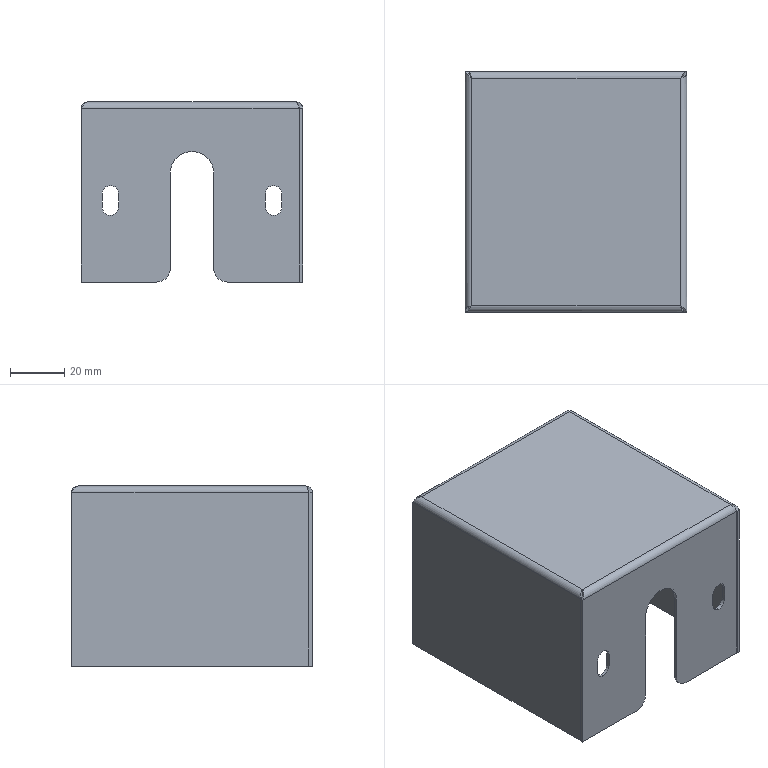Part | SolidWorks | features ICE 3, CornerFeat 1, EdgeFlange 1, Fillet 1, FlatPattern 1, SMBaseFlange 1, SheetMetal 1 | 1 solid | 72 faces | box 81.4 x 88.4 x 66.2 mm | volume 32314 mm3 | plane 36 | cylinder 28 | spline 8 | commonest cylinder face diameters 6 x12 2.4 x4 4.8 x4 10 x4 16 x4